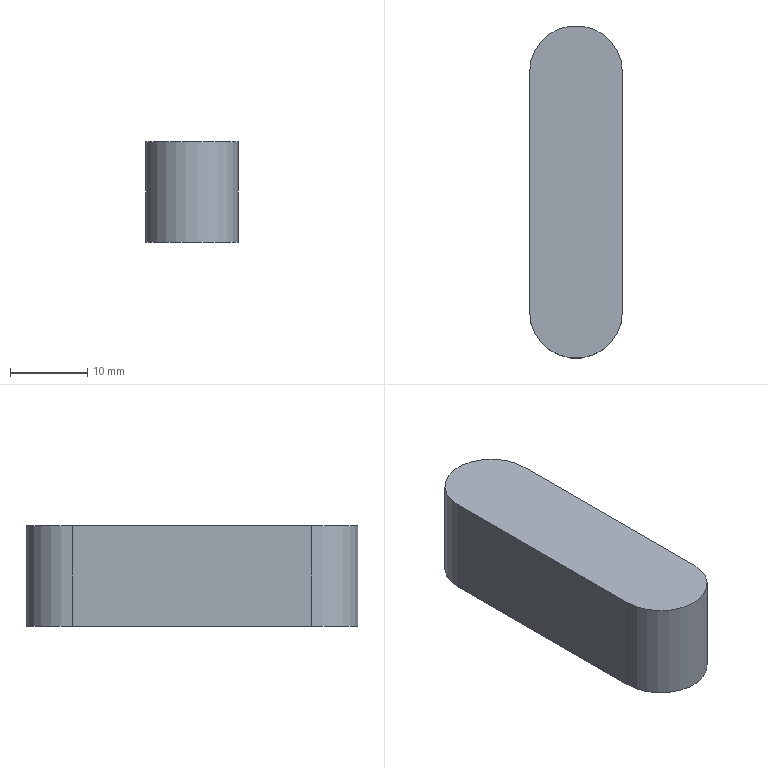Part | NX | features DATUM_CSYS 2, BLEND 1, EXTRUDE 1, OFFSET_REGION 1, SKETCH 1 | 1 solid | 6 faces | box 12 x 43 x 13 mm | volume 6306 mm3 | plane 4 | cylinder 2 | commonest cylinder face diameters 12 x2
STEP:
#1=CARTESIAN_POINT('',(-6.,15.5,13.));
#2=VERTEX_POINT('',#1);
#3=CARTESIAN_POINT('',(-6.,-15.5,13.));
#4=VERTEX_POINT('',#3);
#5=CARTESIAN_POINT('',(-6.,21.5,13.));
#6=DIRECTION('',(0.,-1.,0.));
#7=VECTOR('',#6,1000.);
#8=LINE('',#5,#7);
#9=EDGE_CURVE('',#2,#4,#8,.T.);
#10=ORIENTED_EDGE('',*,*,#9,.F.);
#11=CARTESIAN_POINT('',(-6.,15.5,0.));
#12=VERTEX_POINT('',#11);
#13=CARTESIAN_POINT('',(-6.,15.5,8.));
#14=DIRECTION('',(0.,0.,-1.));
#15=VECTOR('',#14,1000.);
#16=LINE('',#13,#15);
#17=EDGE_CURVE('',#2,#12,#16,.T.);
#18=ORIENTED_EDGE('',*,*,#17,.T.);
#19=CARTESIAN_POINT('',(-6.,-15.5,0.));
#20=VERTEX_POINT('',#19);
#21=CARTESIAN_POINT('',(-6.,21.5,0.));
#22=DIRECTION('',(0.,-1.,0.));
#23=VECTOR('',#22,1000.);
#24=LINE('',#21,#23);
#25=EDGE_CURVE('',#12,#20,#24,.T.);
#26=ORIENTED_EDGE('',*,*,#25,.T.);
#27=CARTESIAN_POINT('',(-6.,-15.5,8.));
#28=DIRECTION('',(0.,0.,-1.));
#29=VECTOR('',#28,1000.);
#30=LINE('',#27,#29);
#31=EDGE_CURVE('',#20,#4,#30,.F.);
#32=ORIENTED_EDGE('',*,*,#31,.T.);
#33=EDGE_LOOP('',(#10,#18,#26,#32));
#34=FACE_BOUND('',#33,.T.);
#35=CARTESIAN_POINT('',(-6.,21.5,8.));
#36=DIRECTION('',(1.,0.,0.));
#37=DIRECTION('',(0.,0.,-1.));
#38=AXIS2_PLACEMENT_3D('',#35,#36,#37);
#39=PLANE('',#38);
#40=ADVANCED_FACE('',(#34),#39,.F.);
#41=CARTESIAN_POINT('',(6.,-15.5,0.));
#42=VERTEX_POINT('',#41);
#43=CARTESIAN_POINT('',(6.,15.5,0.));
#44=VERTEX_POINT('',#43);
#45=CARTESIAN_POINT('',(6.,-21.5,0.));
#46=DIRECTION('',(0.,1.,0.));
#47=VECTOR('',#46,1000.);
#48=LINE('',#45,#47);
#49=EDGE_CURVE('',#42,#44,#48,.T.);
#50=ORIENTED_EDGE('',*,*,#49,.T.);
#51=CARTESIAN_POINT('',(6.,15.5,13.));
#52=VERTEX_POINT('',#51);
#53=CARTESIAN_POINT('',(6.,15.5,8.));
#54=DIRECTION('',(0.,0.,-1.));
#55=VECTOR('',#54,1000.);
#56=LINE('',#53,#55);
#57=EDGE_CURVE('',#44,#52,#56,.F.);
#58=ORIENTED_EDGE('',*,*,#57,.T.);
#59=CARTESIAN_POINT('',(6.,-15.5,13.));
#60=VERTEX_POINT('',#59);
#61=CARTESIAN_POINT('',(6.,-21.5,13.));
#62=DIRECTION('',(0.,1.,0.));
#63=VECTOR('',#62,1000.);
#64=LINE('',#61,#63);
#65=EDGE_CURVE('',#60,#52,#64,.T.);
#66=ORIENTED_EDGE('',*,*,#65,.F.);
#67=CARTESIAN_POINT('',(6.,-15.5,8.));
#68=DIRECTION('',(0.,0.,-1.));
#69=VECTOR('',#68,1000.);
#70=LINE('',#67,#69);
#71=EDGE_CURVE('',#60,#42,#70,.T.);
#72=ORIENTED_EDGE('',*,*,#71,.T.);
#73=EDGE_LOOP('',(#50,#58,#66,#72));
#74=FACE_BOUND('',#73,.T.);
#75=CARTESIAN_POINT('',(6.,-21.5,8.));
#76=DIRECTION('',(-1.,0.,0.));
#77=DIRECTION('',(0.,0.,1.));
#78=AXIS2_PLACEMENT_3D('',#75,#76,#77);
#79=PLANE('',#78);
#80=ADVANCED_FACE('',(#74),#79,.F.);
#81=CARTESIAN_POINT('',(0.,15.5,13.));
#82=DIRECTION('',(0.,0.,1.));
#83=DIRECTION('',(1.,0.,0.));
#84=AXIS2_PLACEMENT_3D('',#81,#82,#83);
#85=CIRCLE('',#84,6.);
#86=EDGE_CURVE('',#52,#2,#85,.T.);
#87=ORIENTED_EDGE('',*,*,#86,.T.);
#88=ORIENTED_EDGE('',*,*,#9,.T.);
#89=CARTESIAN_POINT('',(0.,-15.5,13.));
#90=DIRECTION('',(0.,0.,1.));
#91=DIRECTION('',(1.,0.,0.));
#92=AXIS2_PLACEMENT_3D('',#89,#90,#91);
#93=CIRCLE('',#92,6.);
#94=EDGE_CURVE('',#4,#60,#93,.T.);
#95=ORIENTED_EDGE('',*,*,#94,.T.);
#96=ORIENTED_EDGE('',*,*,#65,.T.);
#97=EDGE_LOOP('',(#87,#88,#95,#96));
#98=FACE_BOUND('',#97,.T.);
#99=CARTESIAN_POINT('',(0.,0.,13.));
#100=DIRECTION('',(0.,0.,1.));
#101=DIRECTION('',(1.,0.,0.));
#102=AXIS2_PLACEMENT_3D('',#99,#100,#101);
#103=PLANE('',#102);
#104=ADVANCED_FACE('',(#98),#103,.T.);
#105=ORIENTED_EDGE('',*,*,#25,.F.);
#106=CARTESIAN_POINT('',(0.,15.5,0.));
#107=DIRECTION('',(0.,0.,1.));
#108=DIRECTION('',(1.,0.,0.));
#109=AXIS2_PLACEMENT_3D('',#106,#107,#108);
#110=CIRCLE('',#109,6.);
#111=EDGE_CURVE('',#12,#44,#110,.F.);
#112=ORIENTED_EDGE('',*,*,#111,.T.);
#113=ORIENTED_EDGE('',*,*,#49,.F.);
#114=CARTESIAN_POINT('',(0.,-15.5,0.));
#115=DIRECTION('',(0.,0.,1.));
#116=DIRECTION('',(1.,0.,0.));
#117=AXIS2_PLACEMENT_3D('',#114,#115,#116);
#118=CIRCLE('',#117,6.);
#119=EDGE_CURVE('',#42,#20,#118,.F.);
#120=ORIENTED_EDGE('',*,*,#119,.T.);
#121=EDGE_LOOP('',(#105,#112,#113,#120));
#122=FACE_BOUND('',#121,.T.);
#123=CARTESIAN_POINT('',(0.,0.,0.));
#124=DIRECTION('',(0.,0.,1.));
#125=DIRECTION('',(1.,0.,0.));
#126=AXIS2_PLACEMENT_3D('',#123,#124,#125);
#127=PLANE('',#126);
#128=ADVANCED_FACE('',(#122),#127,.F.);
#129=ORIENTED_EDGE('',*,*,#111,.F.);
#130=ORIENTED_EDGE('',*,*,#17,.F.);
#131=ORIENTED_EDGE('',*,*,#86,.F.);
#132=ORIENTED_EDGE('',*,*,#57,.F.);
#133=EDGE_LOOP('',(#129,#130,#131,#132));
#134=FACE_BOUND('',#133,.T.);
#135=CARTESIAN_POINT('',(0.,15.5,8.));
#136=DIRECTION('',(0.,0.,-1.));
#137=DIRECTION('',(-1.,0.,0.));
#138=AXIS2_PLACEMENT_3D('',#135,#136,#137);
#139=CYLINDRICAL_SURFACE('',#138,6.);
#140=ADVANCED_FACE('',(#134),#139,.T.);
#141=ORIENTED_EDGE('',*,*,#71,.F.);
#142=ORIENTED_EDGE('',*,*,#94,.F.);
#143=ORIENTED_EDGE('',*,*,#31,.F.);
#144=ORIENTED_EDGE('',*,*,#119,.F.);
#145=EDGE_LOOP('',(#141,#142,#143,#144));
#146=FACE_BOUND('',#145,.T.);
#147=CARTESIAN_POINT('',(0.,-15.5,8.));
#148=DIRECTION('',(0.,0.,-1.));
#149=DIRECTION('',(-1.,0.,0.));
#150=AXIS2_PLACEMENT_3D('',#147,#148,#149);
#151=CYLINDRICAL_SURFACE('',#150,6.);
#152=ADVANCED_FACE('',(#146),#151,.T.);
#153=CLOSED_SHELL('',(#40,#80,#104,#128,#140,#152));
#154=MANIFOLD_SOLID_BREP('',#153);
#155=(LENGTH_UNIT()NAMED_UNIT(*)SI_UNIT(.MILLI.,.METRE.));
#156=UNCERTAINTY_MEASURE_WITH_UNIT(LENGTH_MEASURE(0.00001),#155,'','');
#157=(NAMED_UNIT(*)PLANE_ANGLE_UNIT()SI_UNIT($,.RADIAN.));
#158=(NAMED_UNIT(*)SI_UNIT($,.STERADIAN.)SOLID_ANGLE_UNIT());
#159=(GEOMETRIC_REPRESENTATION_CONTEXT(3)GLOBAL_UNCERTAINTY_ASSIGNED_CONTEXT((#156))GLOBAL_UNIT_ASSIGNED_CONTEXT((#155,#157,#158))REPRESENTATION_CONTEXT('',''));
#160=ADVANCED_BREP_SHAPE_REPRESENTATION('',(#154),#159);